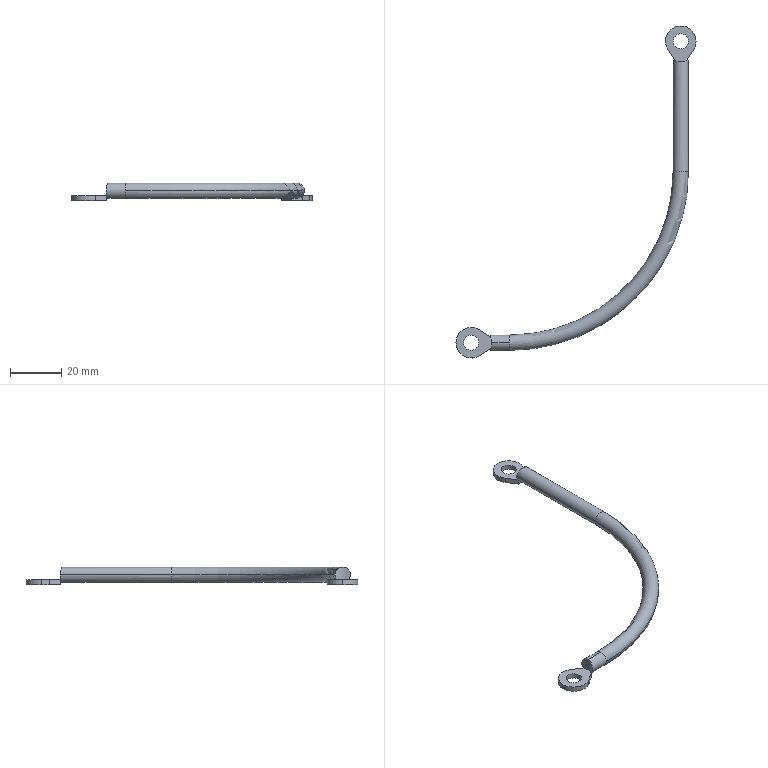Part | SolidWorks | features BaseBody 1 | 1 solid | 27 faces | box 94 x 130 x 7 mm | volume 4790 mm3 | cylinder 15 | plane 10 | torus 2 | commonest cylinder face diameters 6 x8 12 x5 16 x2
STEP:
#1=CARTESIAN_POINT('',(7.681,2.236,-4.));
#2=VERTEX_POINT('',#1);
#3=CARTESIAN_POINT('',(7.681,2.236,-2.));
#4=VERTEX_POINT('',#3);
#5=CARTESIAN_POINT('',(7.681,2.236,-15.078));
#6=DIRECTION('',(0.,0.,1.));
#7=VECTOR('',#6,1000.);
#8=LINE('',#5,#7);
#9=EDGE_CURVE('',#2,#4,#8,.T.);
#10=ORIENTED_EDGE('',*,*,#9,.F.);
#11=CARTESIAN_POINT('',(3.211,5.068,-4.));
#12=VERTEX_POINT('',#11);
#13=CARTESIAN_POINT('',(3.211,5.068,-4.));
#14=DIRECTION('',(-0.8447,0.5352,0.));
#15=VECTOR('',#14,1000.);
#16=LINE('',#13,#15);
#17=EDGE_CURVE('',#2,#12,#16,.T.);
#18=ORIENTED_EDGE('',*,*,#17,.T.);
#19=CARTESIAN_POINT('',(3.211,5.068,-2.));
#20=VERTEX_POINT('',#19);
#21=CARTESIAN_POINT('',(3.211,5.068,-15.078));
#22=DIRECTION('',(0.,0.,1.));
#23=VECTOR('',#22,1000.);
#24=LINE('',#21,#23);
#25=EDGE_CURVE('',#12,#20,#24,.T.);
#26=ORIENTED_EDGE('',*,*,#25,.T.);
#27=CARTESIAN_POINT('',(3.211,5.068,-2.));
#28=DIRECTION('',(0.8447,-0.5352,0.));
#29=VECTOR('',#28,1000.);
#30=LINE('',#27,#29);
#31=EDGE_CURVE('',#20,#4,#30,.T.);
#32=ORIENTED_EDGE('',*,*,#31,.T.);
#33=EDGE_LOOP('',(#10,#18,#26,#32));
#34=FACE_OUTER_BOUND('',#33,.T.);
#35=CARTESIAN_POINT('',(3.211,5.068,-15.078));
#36=DIRECTION('',(-0.5352,-0.8447,0.));
#37=DIRECTION('',(-0.8447,0.5352,0.));
#38=AXIS2_PLACEMENT_3D('',#35,#36,#37);
#39=PLANE('',#38);
#40=ADVANCED_FACE('',(#34),#39,.F.);
#41=CARTESIAN_POINT('',(7.681,-2.236,-2.));
#42=VERTEX_POINT('',#41);
#43=CARTESIAN_POINT('',(7.681,0.,-3.));
#44=VERTEX_POINT('',#43);
#45=CARTESIAN_POINT('',(7.681,0.,0.));
#46=DIRECTION('',(1.,0.,0.));
#47=DIRECTION('',(0.,0.,1.));
#48=AXIS2_PLACEMENT_3D('',#45,#46,#47);
#49=CIRCLE('',#48,3.);
#50=EDGE_CURVE('',#42,#44,#49,.T.);
#51=ORIENTED_EDGE('',*,*,#50,.F.);
#52=CARTESIAN_POINT('',(7.681,-2.236,-4.));
#53=VERTEX_POINT('',#52);
#54=CARTESIAN_POINT('',(7.681,-2.236,-15.078));
#55=DIRECTION('',(0.,0.,1.));
#56=VECTOR('',#55,1000.);
#57=LINE('',#54,#56);
#58=EDGE_CURVE('',#53,#42,#57,.T.);
#59=ORIENTED_EDGE('',*,*,#58,.F.);
#60=CARTESIAN_POINT('',(7.681,2.236,-4.));
#61=DIRECTION('',(0.,1.,0.));
#62=VECTOR('',#61,1000.);
#63=LINE('',#60,#62);
#64=EDGE_CURVE('',#53,#2,#63,.T.);
#65=ORIENTED_EDGE('',*,*,#64,.T.);
#66=ORIENTED_EDGE('',*,*,#9,.T.);
#67=CARTESIAN_POINT('',(7.681,0.,0.));
#68=DIRECTION('',(1.,0.,0.));
#69=DIRECTION('',(0.,0.,1.));
#70=AXIS2_PLACEMENT_3D('',#67,#68,#69);
#71=CIRCLE('',#70,3.);
#72=EDGE_CURVE('',#44,#4,#71,.T.);
#73=ORIENTED_EDGE('',*,*,#72,.F.);
#74=EDGE_LOOP('',(#51,#59,#65,#66,#73));
#75=FACE_OUTER_BOUND('',#74,.T.);
#76=CARTESIAN_POINT('',(7.681,2.236,-15.078));
#77=DIRECTION('',(-1.,0.,0.));
#78=DIRECTION('',(0.,0.,1.));
#79=AXIS2_PLACEMENT_3D('',#76,#77,#78);
#80=PLANE('',#79);
#81=ADVANCED_FACE('',(#75),#80,.F.);
#82=CARTESIAN_POINT('',(3.211,-5.068,-4.));
#83=VERTEX_POINT('',#82);
#84=CARTESIAN_POINT('',(3.211,-5.068,-2.));
#85=VERTEX_POINT('',#84);
#86=CARTESIAN_POINT('',(3.211,-5.068,-15.078));
#87=DIRECTION('',(0.,0.,1.));
#88=VECTOR('',#87,1000.);
#89=LINE('',#86,#88);
#90=EDGE_CURVE('',#83,#85,#89,.T.);
#91=ORIENTED_EDGE('',*,*,#90,.F.);
#92=CARTESIAN_POINT('',(7.681,-2.236,-4.));
#93=DIRECTION('',(0.8447,0.5352,0.));
#94=VECTOR('',#93,1000.);
#95=LINE('',#92,#94);
#96=EDGE_CURVE('',#83,#53,#95,.T.);
#97=ORIENTED_EDGE('',*,*,#96,.T.);
#98=ORIENTED_EDGE('',*,*,#58,.T.);
#99=CARTESIAN_POINT('',(7.681,-2.236,-2.));
#100=DIRECTION('',(-0.8447,-0.5352,0.));
#101=VECTOR('',#100,1000.);
#102=LINE('',#99,#101);
#103=EDGE_CURVE('',#42,#85,#102,.T.);
#104=ORIENTED_EDGE('',*,*,#103,.T.);
#105=EDGE_LOOP('',(#91,#97,#98,#104));
#106=FACE_OUTER_BOUND('',#105,.T.);
#107=CARTESIAN_POINT('',(7.681,-2.236,-15.078));
#108=DIRECTION('',(-0.5352,0.8447,0.));
#109=DIRECTION('',(0.,0.,1.));
#110=AXIS2_PLACEMENT_3D('',#107,#108,#109);
#111=PLANE('',#110);
#112=ADVANCED_FACE('',(#106),#111,.F.);
#113=CARTESIAN_POINT('',(84.236,110.319,-4.));
#114=VERTEX_POINT('',#113);
#115=CARTESIAN_POINT('',(84.236,110.319,-2.));
#116=VERTEX_POINT('',#115);
#117=CARTESIAN_POINT('',(84.236,110.319,-15.078));
#118=DIRECTION('',(0.,0.,1.));
#119=VECTOR('',#118,1000.);
#120=LINE('',#117,#119);
#121=EDGE_CURVE('',#114,#116,#120,.T.);
#122=ORIENTED_EDGE('',*,*,#121,.F.);
#123=CARTESIAN_POINT('',(87.068,114.789,-4.));
#124=VERTEX_POINT('',#123);
#125=CARTESIAN_POINT('',(87.068,114.789,-4.));
#126=DIRECTION('',(0.5352,0.8447,0.));
#127=VECTOR('',#126,1000.);
#128=LINE('',#125,#127);
#129=EDGE_CURVE('',#114,#124,#128,.T.);
#130=ORIENTED_EDGE('',*,*,#129,.T.);
#131=CARTESIAN_POINT('',(87.068,114.789,-2.));
#132=VERTEX_POINT('',#131);
#133=CARTESIAN_POINT('',(87.068,114.789,-15.078));
#134=DIRECTION('',(0.,0.,1.));
#135=VECTOR('',#134,1000.);
#136=LINE('',#133,#135);
#137=EDGE_CURVE('',#124,#132,#136,.T.);
#138=ORIENTED_EDGE('',*,*,#137,.T.);
#139=CARTESIAN_POINT('',(87.068,114.789,-2.));
#140=DIRECTION('',(-0.5352,-0.8447,0.));
#141=VECTOR('',#140,1000.);
#142=LINE('',#139,#141);
#143=EDGE_CURVE('',#132,#116,#142,.T.);
#144=ORIENTED_EDGE('',*,*,#143,.T.);
#145=EDGE_LOOP('',(#122,#130,#138,#144));
#146=FACE_OUTER_BOUND('',#145,.T.);
#147=CARTESIAN_POINT('',(87.068,114.789,-15.078));
#148=DIRECTION('',(-0.8447,0.5352,0.));
#149=DIRECTION('',(0.,0.,1.));
#150=AXIS2_PLACEMENT_3D('',#147,#148,#149);
#151=PLANE('',#150);
#152=ADVANCED_FACE('',(#146),#151,.F.);
#153=CARTESIAN_POINT('',(79.764,110.319,-2.));
#154=VERTEX_POINT('',#153);
#155=CARTESIAN_POINT('',(82.,110.319,0.));
#156=DIRECTION('',(0.,-1.,0.));
#157=DIRECTION('',(0.,0.,1.));
#158=AXIS2_PLACEMENT_3D('',#155,#156,#157);
#159=CIRCLE('',#158,3.);
#160=EDGE_CURVE('',#154,#116,#159,.T.);
#161=ORIENTED_EDGE('',*,*,#160,.F.);
#162=CARTESIAN_POINT('',(79.764,110.319,-4.));
#163=VERTEX_POINT('',#162);
#164=CARTESIAN_POINT('',(79.764,110.319,-15.078));
#165=DIRECTION('',(0.,0.,1.));
#166=VECTOR('',#165,1000.);
#167=LINE('',#164,#166);
#168=EDGE_CURVE('',#163,#154,#167,.T.);
#169=ORIENTED_EDGE('',*,*,#168,.F.);
#170=CARTESIAN_POINT('',(84.236,110.319,-4.));
#171=DIRECTION('',(1.,0.,0.));
#172=VECTOR('',#171,1000.);
#173=LINE('',#170,#172);
#174=EDGE_CURVE('',#163,#114,#173,.T.);
#175=ORIENTED_EDGE('',*,*,#174,.T.);
#176=ORIENTED_EDGE('',*,*,#121,.T.);
#177=EDGE_LOOP('',(#161,#169,#175,#176));
#178=FACE_OUTER_BOUND('',#177,.T.);
#179=CARTESIAN_POINT('',(84.236,110.319,-15.078));
#180=DIRECTION('',(0.,1.,0.));
#181=DIRECTION('',(1.,0.,0.));
#182=AXIS2_PLACEMENT_3D('',#179,#180,#181);
#183=PLANE('',#182);
#184=ADVANCED_FACE('',(#178),#183,.F.);
#185=CARTESIAN_POINT('',(76.932,114.789,-4.));
#186=VERTEX_POINT('',#185);
#187=CARTESIAN_POINT('',(76.932,114.789,-2.));
#188=VERTEX_POINT('',#187);
#189=CARTESIAN_POINT('',(76.932,114.789,-15.078));
#190=DIRECTION('',(0.,0.,1.));
#191=VECTOR('',#190,1000.);
#192=LINE('',#189,#191);
#193=EDGE_CURVE('',#186,#188,#192,.T.);
#194=ORIENTED_EDGE('',*,*,#193,.F.);
#195=CARTESIAN_POINT('',(79.764,110.319,-4.));
#196=DIRECTION('',(0.5352,-0.8447,0.));
#197=VECTOR('',#196,1000.);
#198=LINE('',#195,#197);
#199=EDGE_CURVE('',#186,#163,#198,.T.);
#200=ORIENTED_EDGE('',*,*,#199,.T.);
#201=ORIENTED_EDGE('',*,*,#168,.T.);
#202=CARTESIAN_POINT('',(79.764,110.319,-2.));
#203=DIRECTION('',(-0.5352,0.8447,0.));
#204=VECTOR('',#203,1000.);
#205=LINE('',#202,#204);
#206=EDGE_CURVE('',#154,#188,#205,.T.);
#207=ORIENTED_EDGE('',*,*,#206,.T.);
#208=EDGE_LOOP('',(#194,#200,#201,#207));
#209=FACE_OUTER_BOUND('',#208,.T.);
#210=CARTESIAN_POINT('',(79.764,110.319,-15.078));
#211=DIRECTION('',(0.8447,0.5352,0.));
#212=DIRECTION('',(0.,0.,-1.));
#213=AXIS2_PLACEMENT_3D('',#210,#211,#212);
#214=PLANE('',#213);
#215=ADVANCED_FACE('',(#209),#214,.F.);
#216=CARTESIAN_POINT('',(0.,0.,-2.));
#217=DIRECTION('',(0.,0.,1.));
#218=DIRECTION('',(1.,0.,0.));
#219=AXIS2_PLACEMENT_3D('',#216,#217,#218);
#220=CIRCLE('',#219,8.);
#221=EDGE_CURVE('',#42,#4,#220,.T.);
#222=ORIENTED_EDGE('',*,*,#221,.F.);
#223=CARTESIAN_POINT('',(8.,0.,3.));
#224=VERTEX_POINT('',#223);
#225=CARTESIAN_POINT('',(8.,0.,3.));
#226=CARTESIAN_POINT('',(8.,-0.1411,3.));
#227=CARTESIAN_POINT('',(7.996,-0.284,2.99));
#228=CARTESIAN_POINT('',(7.985,-0.499,2.959));
#229=CARTESIAN_POINT('',(7.98,-0.5708,2.946));
#230=CARTESIAN_POINT('',(7.971,-0.6783,2.923));
#231=CARTESIAN_POINT('',(7.967,-0.732,2.91));
#232=CARTESIAN_POINT('',(7.96,-0.7945,2.893));
#233=CARTESIAN_POINT('',(7.958,-0.8212,2.885));
#234=CARTESIAN_POINT('',(7.956,-0.839,2.88));
#235=CARTESIAN_POINT('',(7.955,-0.8491,2.877));
#236=CARTESIAN_POINT('',(7.941,-0.9804,2.838));
#237=CARTESIAN_POINT('',(7.924,-1.109,2.791));
#238=CARTESIAN_POINT('',(7.893,-1.305,2.702));
#239=CARTESIAN_POINT('',(7.882,-1.371,2.669));
#240=CARTESIAN_POINT('',(7.864,-1.47,2.615));
#241=CARTESIAN_POINT('',(7.854,-1.52,2.587));
#242=CARTESIAN_POINT('',(7.843,-1.578,2.551));
#243=CARTESIAN_POINT('',(7.837,-1.607,2.533));
#244=CARTESIAN_POINT('',(7.834,-1.62,2.525));
#245=CARTESIAN_POINT('',(7.833,-1.628,2.52));
#246=CARTESIAN_POINT('',(7.832,-1.633,2.516));
#247=CARTESIAN_POINT('',(7.82,-1.687,2.481));
#248=CARTESIAN_POINT('',(7.808,-1.741,2.444));
#249=CARTESIAN_POINT('',(7.789,-1.827,2.38));
#250=CARTESIAN_POINT('',(7.782,-1.856,2.357));
#251=CARTESIAN_POINT('',(7.771,-1.901,2.321));
#252=CARTESIAN_POINT('',(7.765,-1.924,2.302));
#253=CARTESIAN_POINT('',(7.76,-1.947,2.283));
#254=CARTESIAN_POINT('',(7.756,-1.962,2.27));
#255=CARTESIAN_POINT('',(7.753,-1.971,2.262));
#256=CARTESIAN_POINT('',(7.738,-2.031,2.209));
#257=CARTESIAN_POINT('',(7.717,-2.109,2.136));
#258=CARTESIAN_POINT('',(7.693,-2.195,2.046));
#259=CARTESIAN_POINT('',(7.681,-2.237,1.999));
#260=CARTESIAN_POINT('',(7.676,-2.254,1.979));
#261=CARTESIAN_POINT('',(7.672,-2.266,1.966));
#262=CARTESIAN_POINT('',(7.671,-2.271,1.96));
#263=CARTESIAN_POINT('',(7.636,-2.386,1.826));
#264=CARTESIAN_POINT('',(7.608,-2.476,1.7));
#265=CARTESIAN_POINT('',(7.57,-2.589,1.518));
#266=CARTESIAN_POINT('',(7.558,-2.622,1.459));
#267=CARTESIAN_POINT('',(7.542,-2.668,1.371));
#268=CARTESIAN_POINT('',(7.534,-2.69,1.329));
#269=CARTESIAN_POINT('',(7.526,-2.713,1.28));
#270=CARTESIAN_POINT('',(7.522,-2.723,1.259));
#271=CARTESIAN_POINT('',(7.52,-2.729,1.245));
#272=CARTESIAN_POINT('',(7.519,-2.732,1.24));
#273=CARTESIAN_POINT('',(7.495,-2.799,1.091));
#274=CARTESIAN_POINT('',(7.476,-2.849,0.9501));
#275=CARTESIAN_POINT('',(7.453,-2.908,0.7416));
#276=CARTESIAN_POINT('',(7.446,-2.924,0.6726));
#277=CARTESIAN_POINT('',(7.438,-2.946,0.5701));
#278=CARTESIAN_POINT('',(7.434,-2.955,0.5191));
#279=CARTESIAN_POINT('',(7.431,-2.963,0.4685));
#280=CARTESIAN_POINT('',(7.429,-2.968,0.435));
#281=CARTESIAN_POINT('',(7.428,-2.971,0.4194));
#282=CARTESIAN_POINT('',(7.419,-2.992,0.2582));
#283=CARTESIAN_POINT('',(7.416,-3.001,0.1133));
#284=CARTESIAN_POINT('',(7.417,-2.999,-0.1042));
#285=CARTESIAN_POINT('',(7.418,-2.996,-0.1767));
#286=CARTESIAN_POINT('',(7.422,-2.987,-0.2852));
#287=CARTESIAN_POINT('',(7.424,-2.981,-0.3393));
#288=CARTESIAN_POINT('',(7.427,-2.974,-0.3934));
#289=CARTESIAN_POINT('',(7.429,-2.969,-0.4293));
#290=CARTESIAN_POINT('',(7.43,-2.966,-0.4488));
#291=CARTESIAN_POINT('',(7.439,-2.943,-0.5972));
#292=CARTESIAN_POINT('',(7.451,-2.913,-0.733));
#293=CARTESIAN_POINT('',(7.475,-2.85,-0.94));
#294=CARTESIAN_POINT('',(7.484,-2.826,-1.009));
#295=CARTESIAN_POINT('',(7.499,-2.786,-1.114));
#296=CARTESIAN_POINT('',(7.507,-2.764,-1.166));
#297=CARTESIAN_POINT('',(7.517,-2.737,-1.228));
#298=CARTESIAN_POINT('',(7.522,-2.723,-1.258));
#299=CARTESIAN_POINT('',(7.524,-2.717,-1.271));
#300=CARTESIAN_POINT('',(7.526,-2.713,-1.28));
#301=CARTESIAN_POINT('',(7.527,-2.71,-1.286));
#302=CARTESIAN_POINT('',(7.56,-2.618,-1.48));
#303=CARTESIAN_POINT('',(7.611,-2.476,-1.732));
#304=CARTESIAN_POINT('',(7.681,-2.236,-2.));
#305=B_SPLINE_CURVE_WITH_KNOTS('',3,(#225,#226,#227,#228,#229,#230,#231,#232,#233,#234,#235,#236,#237,#238,#239,#240,#241,#242,#243,#244,#245,#246,#247,#248,#249,#250,#251,#252,#253,#254,#255,#256,#257,#258,#259,#260,#261,#262,#263,#264,#265,#266,#267,#268,#269,#270,#271,#272,#273,#274,#275,#276,#277,#278,#279,#280,#281,#282,#283,#284,#285,#286,#287,#288,#289,#290,#291,#292,#293,#294,#295,#296,#297,#298,#299,#300,#301,#302,#303,#304),.UNSPECIFIED.,.F.,.F.,(4,2,2,1,1,2,2,2,2,1,1,1,2,2,2,2,1,2,2,1,1,1,2,2,2,2,1,1,2,2,2,2,1,2,2,2,2,1,2,2,2,2,1,1,1,2,2,4),(0.,0.0625,0.09375,0.1094,0.1172,0.1211,0.125,0.1875,0.2187,0.2344,0.2422,0.2461,0.248,0.25,0.2812,0.2969,0.3047,0.3086,0.3125,0.3437,0.3594,0.3672,0.3711,0.375,0.4375,0.4687,0.4844,0.4922,0.4961,0.5,0.5625,0.5937,0.6094,0.6172,0.625,0.6875,0.7187,0.7344,0.7422,0.75,0.8125,0.8437,0.8594,0.8672,0.8711,0.873,0.875,1.),.UNSPECIFIED.);
#306=EDGE_CURVE('',#224,#42,#305,.T.);
#307=ORIENTED_EDGE('',*,*,#306,.F.);
#308=CARTESIAN_POINT('',(7.681,2.236,-2.));
#309=CARTESIAN_POINT('',(7.646,2.356,-1.866));
#310=CARTESIAN_POINT('',(7.616,2.452,-1.735));
#311=CARTESIAN_POINT('',(7.577,2.567,-1.554));
#312=CARTESIAN_POINT('',(7.566,2.601,-1.497));
#313=CARTESIAN_POINT('',(7.55,2.646,-1.415));
#314=CARTESIAN_POINT('',(7.543,2.667,-1.375));
#315=CARTESIAN_POINT('',(7.535,2.689,-1.331));
#316=CARTESIAN_POINT('',(7.531,2.699,-1.309));
#317=CARTESIAN_POINT('',(7.529,2.704,-1.3));
#318=CARTESIAN_POINT('',(7.528,2.706,-1.294));
#319=CARTESIAN_POINT('',(7.528,2.707,-1.293));
#320=CARTESIAN_POINT('',(7.503,2.776,-1.149));
#321=CARTESIAN_POINT('',(7.483,2.829,-1.009));
#322=CARTESIAN_POINT('',(7.459,2.892,-0.8019));
#323=CARTESIAN_POINT('',(7.452,2.91,-0.7335));
#324=CARTESIAN_POINT('',(7.443,2.933,-0.632));
#325=CARTESIAN_POINT('',(7.439,2.943,-0.5815));
#326=CARTESIAN_POINT('',(7.435,2.953,-0.5315));
#327=CARTESIAN_POINT('',(7.433,2.958,-0.4983));
#328=CARTESIAN_POINT('',(7.432,2.961,-0.4832));
#329=CARTESIAN_POINT('',(7.422,2.986,-0.3218));
#330=CARTESIAN_POINT('',(7.417,2.998,-0.1769));
#331=CARTESIAN_POINT('',(7.416,3.001,0.04039));
#332=CARTESIAN_POINT('',(7.417,2.999,0.1128));
#333=CARTESIAN_POINT('',(7.419,2.992,0.2211));
#334=CARTESIAN_POINT('',(7.421,2.988,0.2752));
#335=CARTESIAN_POINT('',(7.423,2.982,0.3292));
#336=CARTESIAN_POINT('',(7.425,2.978,0.3651));
#337=CARTESIAN_POINT('',(7.426,2.975,0.3842));
#338=CARTESIAN_POINT('',(7.434,2.955,0.5349));
#339=CARTESIAN_POINT('',(7.445,2.927,0.6725));
#340=CARTESIAN_POINT('',(7.468,2.868,0.8818));
#341=CARTESIAN_POINT('',(7.477,2.846,0.9521));
#342=CARTESIAN_POINT('',(7.491,2.808,1.058));
#343=CARTESIAN_POINT('',(7.499,2.787,1.111));
#344=CARTESIAN_POINT('',(7.508,2.762,1.172));
#345=CARTESIAN_POINT('',(7.513,2.748,1.203));
#346=CARTESIAN_POINT('',(7.515,2.742,1.217));
#347=CARTESIAN_POINT('',(7.517,2.738,1.225));
#348=CARTESIAN_POINT('',(7.518,2.736,1.231));
#349=CARTESIAN_POINT('',(7.535,2.689,1.334));
#350=CARTESIAN_POINT('',(7.555,2.632,1.447));
#351=CARTESIAN_POINT('',(7.593,2.52,1.63));
#352=CARTESIAN_POINT('',(7.607,2.478,1.693));
#353=CARTESIAN_POINT('',(7.629,2.408,1.79));
#354=CARTESIAN_POINT('',(7.641,2.371,1.838));
#355=CARTESIAN_POINT('',(7.655,2.325,1.896));
#356=CARTESIAN_POINT('',(7.661,2.304,1.921));
#357=CARTESIAN_POINT('',(7.665,2.29,1.938));
#358=CARTESIAN_POINT('',(7.668,2.282,1.948));
#359=CARTESIAN_POINT('',(7.697,2.183,2.062));
#360=CARTESIAN_POINT('',(7.725,2.082,2.164));
#361=CARTESIAN_POINT('',(7.766,1.923,2.304));
#362=CARTESIAN_POINT('',(7.779,1.868,2.349));
#363=CARTESIAN_POINT('',(7.799,1.782,2.413));
#364=CARTESIAN_POINT('',(7.809,1.739,2.445));
#365=CARTESIAN_POINT('',(7.818,1.695,2.475));
#366=CARTESIAN_POINT('',(7.825,1.665,2.495));
#367=CARTESIAN_POINT('',(7.828,1.652,2.504));
#368=CARTESIAN_POINT('',(7.859,1.503,2.601));
#369=CARTESIAN_POINT('',(7.883,1.37,2.673));
#370=CARTESIAN_POINT('',(7.914,1.174,2.762));
#371=CARTESIAN_POINT('',(7.923,1.109,2.788));
#372=CARTESIAN_POINT('',(7.936,1.013,2.824));
#373=CARTESIAN_POINT('',(7.942,0.9659,2.841));
#374=CARTESIAN_POINT('',(7.948,0.9112,2.858));
#375=CARTESIAN_POINT('',(7.951,0.8879,2.866));
#376=CARTESIAN_POINT('',(7.952,0.8724,2.87));
#377=CARTESIAN_POINT('',(7.953,0.8659,2.872));
#378=CARTESIAN_POINT('',(7.985,0.5721,2.96));
#379=CARTESIAN_POINT('',(8.,0.2822,3.));
#380=CARTESIAN_POINT('',(8.,0.,3.));
#381=B_SPLINE_CURVE_WITH_KNOTS('',3,(#308,#309,#310,#311,#312,#313,#314,#315,#316,#317,#318,#319,#320,#321,#322,#323,#324,#325,#326,#327,#328,#329,#330,#331,#332,#333,#334,#335,#336,#337,#338,#339,#340,#341,#342,#343,#344,#345,#346,#347,#348,#349,#350,#351,#352,#353,#354,#355,#356,#357,#358,#359,#360,#361,#362,#363,#364,#365,#366,#367,#368,#369,#370,#371,#372,#373,#374,#375,#376,#377,#378,#379,#380),.UNSPECIFIED.,.F.,.F.,(4,2,2,1,1,1,2,2,2,2,1,2,2,2,2,1,2,2,2,2,1,1,1,2,2,2,2,1,1,2,2,2,2,1,2,2,2,2,1,1,2,2,4),(0.,0.0625,0.09375,0.1094,0.1172,0.1211,0.123,0.125,0.1875,0.2188,0.2344,0.2422,0.25,0.3125,0.3438,0.3594,0.3672,0.375,0.4375,0.4688,0.4844,0.4922,0.4961,0.498,0.5,0.5625,0.5938,0.6094,0.6172,0.6211,0.625,0.6875,0.7188,0.7344,0.7422,0.75,0.8125,0.8438,0.8594,0.8672,0.8711,0.875,1.),.UNSPECIFIED.);
#382=EDGE_CURVE('',#4,#224,#381,.T.);
#383=ORIENTED_EDGE('',*,*,#382,.F.);
#384=EDGE_LOOP('',(#222,#307,#383));
#385=FACE_OUTER_BOUND('',#384,.T.);
#386=CARTESIAN_POINT('',(0.,0.,13.));
#387=DIRECTION('',(0.,0.,-1.));
#388=DIRECTION('',(-1.,0.,0.));
#389=AXIS2_PLACEMENT_3D('',#386,#387,#388);
#390=CYLINDRICAL_SURFACE('',#389,8.);
#391=ADVANCED_FACE('',(#385),#390,.F.);
#392=CARTESIAN_POINT('',(82.,118.,-2.));
#393=DIRECTION('',(0.,0.,1.));
#394=DIRECTION('',(1.,0.,0.));
#395=AXIS2_PLACEMENT_3D('',#392,#393,#394);
#396=CIRCLE('',#395,8.);
#397=EDGE_CURVE('',#154,#116,#396,.T.);
#398=ORIENTED_EDGE('',*,*,#397,.F.);
#399=CARTESIAN_POINT('',(79.,110.584,0.));
#400=VERTEX_POINT('',#399);
#401=CARTESIAN_POINT('',(79.,110.584,0.));
#402=CARTESIAN_POINT('',(79.,110.584,-0.1738));
#403=CARTESIAN_POINT('',(79.015,110.577,-0.3525));
#404=CARTESIAN_POINT('',(79.064,110.558,-0.6234));
#405=CARTESIAN_POINT('',(79.085,110.55,-0.7141));
#406=CARTESIAN_POINT('',(79.123,110.535,-0.8502));
#407=CARTESIAN_POINT('',(79.143,110.527,-0.9182));
#408=CARTESIAN_POINT('',(79.17,110.517,-0.9974));
#409=CARTESIAN_POINT('',(79.183,110.512,-1.031));
#410=CARTESIAN_POINT('',(79.191,110.509,-1.054));
#411=CARTESIAN_POINT('',(79.196,110.507,-1.067));
#412=CARTESIAN_POINT('',(79.229,110.495,-1.154));
#413=CARTESIAN_POINT('',(79.264,110.482,-1.233));
#414=CARTESIAN_POINT('',(79.323,110.461,-1.356));
#415=CARTESIAN_POINT('',(79.355,110.45,-1.417));
#416=CARTESIAN_POINT('',(79.396,110.436,-1.49));
#417=CARTESIAN_POINT('',(79.418,110.428,-1.527));
#418=CARTESIAN_POINT('',(79.427,110.425,-1.543));
#419=CARTESIAN_POINT('',(79.434,110.423,-1.553));
#420=CARTESIAN_POINT('',(79.438,110.421,-1.56));
#421=CARTESIAN_POINT('',(79.512,110.396,-1.682));
#422=CARTESIAN_POINT('',(79.615,110.362,-1.833));
#423=CARTESIAN_POINT('',(79.764,110.319,-2.));
#424=B_SPLINE_CURVE_WITH_KNOTS('',3,(#401,#402,#403,#404,#405,#406,#407,#408,#409,#410,#411,#412,#413,#414,#415,#416,#417,#418,#419,#420,#421,#422,#423),.UNSPECIFIED.,.F.,.F.,(4,2,2,1,1,2,2,2,1,1,1,2,2,4),(0.,0.25,0.375,0.4375,0.4688,0.4844,0.5,0.625,0.6875,0.7188,0.7344,0.7422,0.75,1.),.UNSPECIFIED.);
#425=EDGE_CURVE('',#400,#154,#424,.T.);
#426=ORIENTED_EDGE('',*,*,#425,.F.);
#427=CARTESIAN_POINT('',(85.,110.584,0.));
#428=VERTEX_POINT('',#427);
#429=CARTESIAN_POINT('',(85.,110.584,0.));
#430=CARTESIAN_POINT('',(85.,110.584,0.1858));
#431=CARTESIAN_POINT('',(84.983,110.576,0.3779));
#432=CARTESIAN_POINT('',(84.926,110.554,0.6697));
#433=CARTESIAN_POINT('',(84.902,110.544,0.7675));
#434=CARTESIAN_POINT('',(84.858,110.528,0.9143));
#435=CARTESIAN_POINT('',(84.834,110.519,0.9876));
#436=CARTESIAN_POINT('',(84.802,110.507,1.073));
#437=CARTESIAN_POINT('',(84.785,110.5,1.116));
#438=CARTESIAN_POINT('',(84.776,110.497,1.137));
#439=CARTESIAN_POINT('',(84.773,110.496,1.146));
#440=CARTESIAN_POINT('',(84.77,110.495,1.152));
#441=CARTESIAN_POINT('',(84.768,110.494,1.156));
#442=CARTESIAN_POINT('',(84.72,110.476,1.273));
#443=CARTESIAN_POINT('',(84.651,110.45,1.417));
#444=CARTESIAN_POINT('',(84.497,110.398,1.666));
#445=CARTESIAN_POINT('',(84.437,110.379,1.754));
#446=CARTESIAN_POINT('',(84.331,110.346,1.89));
#447=CARTESIAN_POINT('',(84.293,110.335,1.936));
#448=CARTESIAN_POINT('',(84.231,110.317,2.006));
#449=CARTESIAN_POINT('',(84.21,110.311,2.029));
#450=CARTESIAN_POINT('',(84.166,110.299,2.076));
#451=CARTESIAN_POINT('',(84.142,110.292,2.101));
#452=CARTESIAN_POINT('',(83.943,110.237,2.299));
#453=CARTESIAN_POINT('',(83.764,110.196,2.434));
#454=CARTESIAN_POINT('',(83.517,110.146,2.59));
#455=CARTESIAN_POINT('',(83.438,110.131,2.634));
#456=CARTESIAN_POINT('',(83.326,110.111,2.691));
#457=CARTESIAN_POINT('',(83.29,110.105,2.709));
#458=CARTESIAN_POINT('',(83.238,110.096,2.733));
#459=CARTESIAN_POINT('',(83.212,110.092,2.744));
#460=CARTESIAN_POINT('',(83.183,110.088,2.757));
#461=CARTESIAN_POINT('',(83.171,110.086,2.762));
#462=CARTESIAN_POINT('',(83.162,110.085,2.766));
#463=CARTESIAN_POINT('',(83.16,110.085,2.767));
#464=CARTESIAN_POINT('',(82.772,110.028,2.928));
#465=CARTESIAN_POINT('',(82.377,110.,3.));
#466=CARTESIAN_POINT('',(81.815,110.,3.));
#467=CARTESIAN_POINT('',(81.622,110.007,2.983));
#468=CARTESIAN_POINT('',(81.331,110.028,2.926));
#469=CARTESIAN_POINT('',(81.234,110.036,2.902));
#470=CARTESIAN_POINT('',(81.089,110.052,2.859));
#471=CARTESIAN_POINT('',(81.016,110.061,2.835));
#472=CARTESIAN_POINT('',(80.932,110.072,2.804));
#473=CARTESIAN_POINT('',(80.89,110.077,2.787));
#474=CARTESIAN_POINT('',(80.872,110.08,2.78));
#475=CARTESIAN_POINT('',(80.86,110.082,2.775));
#476=CARTESIAN_POINT('',(80.852,110.083,2.772));
#477=CARTESIAN_POINT('',(80.719,110.102,2.716));
#478=CARTESIAN_POINT('',(80.567,110.129,2.643));
#479=CARTESIAN_POINT('',(80.319,110.179,2.487));
#480=CARTESIAN_POINT('',(80.233,110.198,2.427));
#481=CARTESIAN_POINT('',(80.101,110.229,2.323));
#482=CARTESIAN_POINT('',(80.057,110.24,2.286));
#483=CARTESIAN_POINT('',(79.99,110.257,2.228));
#484=CARTESIAN_POINT('',(79.968,110.262,2.207));
#485=CARTESIAN_POINT('',(79.924,110.274,2.166));
#486=CARTESIAN_POINT('',(79.903,110.28,2.145));
#487=CARTESIAN_POINT('',(79.691,110.338,1.934));
#488=CARTESIAN_POINT('',(79.554,110.381,1.747));
#489=CARTESIAN_POINT('',(79.399,110.433,1.498));
#490=CARTESIAN_POINT('',(79.356,110.448,1.421));
#491=CARTESIAN_POINT('',(79.303,110.468,1.313));
#492=CARTESIAN_POINT('',(79.286,110.474,1.279));
#493=CARTESIAN_POINT('',(79.264,110.482,1.231));
#494=CARTESIAN_POINT('',(79.254,110.486,1.207));
#495=CARTESIAN_POINT('',(79.242,110.49,1.181));
#496=CARTESIAN_POINT('',(79.237,110.492,1.168));
#497=CARTESIAN_POINT('',(79.234,110.493,1.163));
#498=CARTESIAN_POINT('',(79.233,110.494,1.159));
#499=CARTESIAN_POINT('',(79.233,110.494,1.158));
#500=CARTESIAN_POINT('',(79.07,110.554,0.768));
#501=CARTESIAN_POINT('',(79.,110.584,0.3709));
#502=CARTESIAN_POINT('',(79.,110.584,0.));
#503=B_SPLINE_CURVE_WITH_KNOTS('',3,(#429,#430,#431,#432,#433,#434,#435,#436,#437,#438,#439,#440,#441,#442,#443,#444,#445,#446,#447,#448,#449,#450,#451,#452,#453,#454,#455,#456,#457,#458,#459,#460,#461,#462,#463,#464,#465,#466,#467,#468,#469,#470,#471,#472,#473,#474,#475,#476,#477,#478,#479,#480,#481,#482,#483,#484,#485,#486,#487,#488,#489,#490,#491,#492,#493,#494,#495,#496,#497,#498,#499,#500,#501,#502),.UNSPECIFIED.,.F.,.F.,(4,2,2,1,1,1,1,2,2,2,2,2,2,2,2,2,2,1,1,2,2,2,2,2,1,1,1,2,2,2,2,2,2,2,2,2,2,1,1,1,2,2,4),(0.,0.0625,0.09375,0.1094,0.1172,0.1211,0.123,0.124,0.125,0.1875,0.2187,0.2344,0.2422,0.25,0.3125,0.3437,0.3594,0.3672,0.3711,0.373,0.375,0.5,0.5625,0.5937,0.6094,0.6172,0.6211,0.623,0.625,0.6875,0.7187,0.7344,0.7422,0.75,0.8125,0.8437,0.8594,0.8672,0.8711,0.873,0.874,0.875,1.),.UNSPECIFIED.);
#504=EDGE_CURVE('',#428,#400,#503,.T.);
#505=ORIENTED_EDGE('',*,*,#504,.F.);
#506=CARTESIAN_POINT('',(84.236,110.319,-2.));
#507=CARTESIAN_POINT('',(84.31,110.34,-1.918));
#508=CARTESIAN_POINT('',(84.372,110.359,-1.839));
#509=CARTESIAN_POINT('',(84.452,110.385,-1.729));
#510=CARTESIAN_POINT('',(84.476,110.393,-1.694));
#511=CARTESIAN_POINT('',(84.51,110.404,-1.644));
#512=CARTESIAN_POINT('',(84.526,110.409,-1.619));
#513=CARTESIAN_POINT('',(84.543,110.415,-1.591));
#514=CARTESIAN_POINT('',(84.55,110.417,-1.58));
#515=CARTESIAN_POINT('',(84.555,110.419,-1.572));
#516=CARTESIAN_POINT('',(84.556,110.419,-1.57));
#517=CARTESIAN_POINT('',(84.612,110.438,-1.48));
#518=CARTESIAN_POINT('',(84.657,110.454,-1.396));
#519=CARTESIAN_POINT('',(84.717,110.475,-1.273));
#520=CARTESIAN_POINT('',(84.735,110.482,-1.233));
#521=CARTESIAN_POINT('',(84.761,110.492,-1.173));
#522=CARTESIAN_POINT('',(84.774,110.496,-1.144));
#523=CARTESIAN_POINT('',(84.785,110.5,-1.115));
#524=CARTESIAN_POINT('',(84.793,110.503,-1.095));
#525=CARTESIAN_POINT('',(84.796,110.505,-1.087));
#526=CARTESIAN_POINT('',(84.939,110.558,-0.7156));
#527=CARTESIAN_POINT('',(85.,110.584,-0.3475));
#528=CARTESIAN_POINT('',(85.,110.584,0.));
#529=B_SPLINE_CURVE_WITH_KNOTS('',3,(#506,#507,#508,#509,#510,#511,#512,#513,#514,#515,#516,#517,#518,#519,#520,#521,#522,#523,#524,#525,#526,#527,#528),.UNSPECIFIED.,.F.,.F.,(4,2,2,1,1,2,2,2,2,1,2,2,4),(0.,0.125,0.1875,0.2187,0.2344,0.2422,0.25,0.375,0.4375,0.4687,0.4844,0.5,1.),.UNSPECIFIED.);
#530=EDGE_CURVE('',#116,#428,#529,.T.);
#531=ORIENTED_EDGE('',*,*,#530,.F.);
#532=EDGE_LOOP('',(#398,#426,#505,#531));
#533=FACE_OUTER_BOUND('',#532,.T.);
#534=CARTESIAN_POINT('',(82.,118.,13.));
#535=DIRECTION('',(0.,0.,-1.));
#536=DIRECTION('',(-1.,0.,0.));
#537=AXIS2_PLACEMENT_3D('',#534,#535,#536);
#538=CYLINDRICAL_SURFACE('',#537,8.);
#539=ADVANCED_FACE('',(#533),#538,.F.);
#540=CARTESIAN_POINT('',(85.,118.,-2.));
#541=VERTEX_POINT('',#540);
#542=CARTESIAN_POINT('',(85.,118.,-4.));
#543=VERTEX_POINT('',#542);
#544=CARTESIAN_POINT('',(85.,118.,1.));
#545=DIRECTION('',(0.,0.,-1.));
#546=VECTOR('',#545,1000.);
#547=LINE('',#544,#546);
#548=EDGE_CURVE('',#541,#543,#547,.T.);
#549=ORIENTED_EDGE('',*,*,#548,.F.);
#550=CARTESIAN_POINT('',(79.,118.,-2.));
#551=VERTEX_POINT('',#550);
#552=CARTESIAN_POINT('',(82.,118.,-2.));
#553=DIRECTION('',(0.,0.,1.));
#554=DIRECTION('',(1.,0.,0.));
#555=AXIS2_PLACEMENT_3D('',#552,#553,#554);
#556=CIRCLE('',#555,3.);
#557=EDGE_CURVE('',#541,#551,#556,.T.);
#558=ORIENTED_EDGE('',*,*,#557,.T.);
#559=CARTESIAN_POINT('',(79.,118.,-4.));
#560=VERTEX_POINT('',#559);
#561=CARTESIAN_POINT('',(79.,118.,1.));
#562=DIRECTION('',(0.,0.,-1.));
#563=VECTOR('',#562,1000.);
#564=LINE('',#561,#563);
#565=EDGE_CURVE('',#551,#560,#564,.T.);
#566=ORIENTED_EDGE('',*,*,#565,.T.);
#567=CARTESIAN_POINT('',(82.,118.,-4.));
#568=DIRECTION('',(0.,0.,1.));
#569=DIRECTION('',(1.,0.,0.));
#570=AXIS2_PLACEMENT_3D('',#567,#568,#569);
#571=CIRCLE('',#570,3.);
#572=EDGE_CURVE('',#543,#560,#571,.T.);
#573=ORIENTED_EDGE('',*,*,#572,.F.);
#574=EDGE_LOOP('',(#549,#558,#566,#573));
#575=FACE_OUTER_BOUND('',#574,.T.);
#576=CARTESIAN_POINT('',(82.,118.,1.));
#577=DIRECTION('',(0.,0.,-1.));
#578=DIRECTION('',(-1.,0.,0.));
#579=AXIS2_PLACEMENT_3D('',#576,#577,#578);
#580=CYLINDRICAL_SURFACE('',#579,3.);
#581=ADVANCED_FACE('',(#575),#580,.F.);
#582=CARTESIAN_POINT('',(82.,118.,-4.));
#583=DIRECTION('',(0.,0.,1.));
#584=DIRECTION('',(1.,0.,0.));
#585=AXIS2_PLACEMENT_3D('',#582,#583,#584);
#586=CIRCLE('',#585,3.);
#587=EDGE_CURVE('',#560,#543,#586,.T.);
#588=ORIENTED_EDGE('',*,*,#587,.T.);
#589=ORIENTED_EDGE('',*,*,#572,.T.);
#590=EDGE_LOOP('',(#588,#589));
#591=FACE_BOUND('',#590,.T.);
#592=ORIENTED_EDGE('',*,*,#199,.F.);
#593=CARTESIAN_POINT('',(76.,118.,-4.));
#594=VERTEX_POINT('',#593);
#595=CARTESIAN_POINT('',(82.,118.,-4.));
#596=DIRECTION('',(0.,0.,1.));
#597=DIRECTION('',(1.,0.,0.));
#598=AXIS2_PLACEMENT_3D('',#595,#596,#597);
#599=CIRCLE('',#598,6.);
#600=EDGE_CURVE('',#594,#186,#599,.T.);
#601=ORIENTED_EDGE('',*,*,#600,.F.);
#602=CARTESIAN_POINT('',(88.,118.,-4.));
#603=VERTEX_POINT('',#602);
#604=CARTESIAN_POINT('',(82.,118.,-4.));
#605=DIRECTION('',(0.,0.,1.));
#606=DIRECTION('',(1.,0.,0.));
#607=AXIS2_PLACEMENT_3D('',#604,#605,#606);
#608=CIRCLE('',#607,6.);
#609=EDGE_CURVE('',#603,#594,#608,.T.);
#610=ORIENTED_EDGE('',*,*,#609,.F.);
#611=CARTESIAN_POINT('',(82.,118.,-4.));
#612=DIRECTION('',(0.,0.,1.));
#613=DIRECTION('',(1.,0.,0.));
#614=AXIS2_PLACEMENT_3D('',#611,#612,#613);
#615=CIRCLE('',#614,6.);
#616=EDGE_CURVE('',#124,#603,#615,.T.);
#617=ORIENTED_EDGE('',*,*,#616,.F.);
#618=ORIENTED_EDGE('',*,*,#129,.F.);
#619=ORIENTED_EDGE('',*,*,#174,.F.);
#620=EDGE_LOOP('',(#592,#601,#610,#617,#618,#619));
#621=FACE_OUTER_BOUND('',#620,.T.);
#622=CARTESIAN_POINT('',(82.,118.,-4.));
#623=DIRECTION('',(0.,0.,1.));
#624=DIRECTION('',(1.,0.,0.));
#625=AXIS2_PLACEMENT_3D('',#622,#623,#624);
#626=PLANE('',#625);
#627=ADVANCED_FACE('',(#591,#621),#626,.F.);
#628=CARTESIAN_POINT('',(82.,118.,-2.));
#629=DIRECTION('',(0.,0.,1.));
#630=DIRECTION('',(1.,0.,0.));
#631=AXIS2_PLACEMENT_3D('',#628,#629,#630);
#632=CIRCLE('',#631,3.);
#633=EDGE_CURVE('',#551,#541,#632,.T.);
#634=ORIENTED_EDGE('',*,*,#633,.F.);
#635=ORIENTED_EDGE('',*,*,#557,.F.);
#636=EDGE_LOOP('',(#634,#635));
#637=FACE_BOUND('',#636,.T.);
#638=ORIENTED_EDGE('',*,*,#397,.T.);
#639=ORIENTED_EDGE('',*,*,#143,.F.);
#640=CARTESIAN_POINT('',(88.,118.,-2.));
#641=VERTEX_POINT('',#640);
#642=CARTESIAN_POINT('',(82.,118.,-2.));
#643=DIRECTION('',(0.,0.,1.));
#644=DIRECTION('',(1.,0.,0.));
#645=AXIS2_PLACEMENT_3D('',#642,#643,#644);
#646=CIRCLE('',#645,6.);
#647=EDGE_CURVE('',#132,#641,#646,.T.);
#648=ORIENTED_EDGE('',*,*,#647,.T.);
#649=CARTESIAN_POINT('',(76.,118.,-2.));
#650=VERTEX_POINT('',#649);
#651=CARTESIAN_POINT('',(82.,118.,-2.));
#652=DIRECTION('',(0.,0.,1.));
#653=DIRECTION('',(1.,0.,0.));
#654=AXIS2_PLACEMENT_3D('',#651,#652,#653);
#655=CIRCLE('',#654,6.);
#656=EDGE_CURVE('',#641,#650,#655,.T.);
#657=ORIENTED_EDGE('',*,*,#656,.T.);
#658=CARTESIAN_POINT('',(82.,118.,-2.));
#659=DIRECTION('',(0.,0.,1.));
#660=DIRECTION('',(1.,0.,0.));
#661=AXIS2_PLACEMENT_3D('',#658,#659,#660);
#662=CIRCLE('',#661,6.);
#663=EDGE_CURVE('',#650,#188,#662,.T.);
#664=ORIENTED_EDGE('',*,*,#663,.T.);
#665=ORIENTED_EDGE('',*,*,#206,.F.);
#666=EDGE_LOOP('',(#638,#639,#648,#657,#664,#665));
#667=FACE_OUTER_BOUND('',#666,.T.);
#668=CARTESIAN_POINT('',(82.,118.,-2.));
#669=DIRECTION('',(0.,0.,1.));
#670=DIRECTION('',(1.,0.,0.));
#671=AXIS2_PLACEMENT_3D('',#668,#669,#670);
#672=PLANE('',#671);
#673=ADVANCED_FACE('',(#637,#667),#672,.T.);
#674=CARTESIAN_POINT('',(3.,0.,-2.));
#675=VERTEX_POINT('',#674);
#676=CARTESIAN_POINT('',(3.,0.,-4.));
#677=VERTEX_POINT('',#676);
#678=CARTESIAN_POINT('',(3.,0.,1.));
#679=DIRECTION('',(0.,0.,-1.));
#680=VECTOR('',#679,1000.);
#681=LINE('',#678,#680);
#682=EDGE_CURVE('',#675,#677,#681,.T.);
#683=ORIENTED_EDGE('',*,*,#682,.F.);
#684=CARTESIAN_POINT('',(-3.,0.,-2.));
#685=VERTEX_POINT('',#684);
#686=CARTESIAN_POINT('',(0.,0.,-2.));
#687=DIRECTION('',(0.,0.,1.));
#688=DIRECTION('',(1.,0.,0.));
#689=AXIS2_PLACEMENT_3D('',#686,#687,#688);
#690=CIRCLE('',#689,3.);
#691=EDGE_CURVE('',#675,#685,#690,.T.);
#692=ORIENTED_EDGE('',*,*,#691,.T.);
#693=CARTESIAN_POINT('',(-3.,0.,-4.));
#694=VERTEX_POINT('',#693);
#695=CARTESIAN_POINT('',(-3.,0.,1.));
#696=DIRECTION('',(0.,0.,-1.));
#697=VECTOR('',#696,1000.);
#698=LINE('',#695,#697);
#699=EDGE_CURVE('',#685,#694,#698,.T.);
#700=ORIENTED_EDGE('',*,*,#699,.T.);
#701=CARTESIAN_POINT('',(0.,0.,-4.));
#702=DIRECTION('',(0.,0.,1.));
#703=DIRECTION('',(1.,0.,0.));
#704=AXIS2_PLACEMENT_3D('',#701,#702,#703);
#705=CIRCLE('',#704,3.);
#706=EDGE_CURVE('',#677,#694,#705,.T.);
#707=ORIENTED_EDGE('',*,*,#706,.F.);
#708=EDGE_LOOP('',(#683,#692,#700,#707));
#709=FACE_OUTER_BOUND('',#708,.T.);
#710=CARTESIAN_POINT('',(0.,0.,1.));
#711=DIRECTION('',(0.,0.,-1.));
#712=DIRECTION('',(-1.,0.,0.));
#713=AXIS2_PLACEMENT_3D('',#710,#711,#712);
#714=CYLINDRICAL_SURFACE('',#713,3.);
#715=ADVANCED_FACE('',(#709),#714,.F.);
#716=CARTESIAN_POINT('',(0.,0.,-4.));
#717=DIRECTION('',(0.,0.,1.));
#718=DIRECTION('',(1.,0.,0.));
#719=AXIS2_PLACEMENT_3D('',#716,#717,#718);
#720=CIRCLE('',#719,3.);
#721=EDGE_CURVE('',#694,#677,#720,.T.);
#722=ORIENTED_EDGE('',*,*,#721,.T.);
#723=ORIENTED_EDGE('',*,*,#706,.T.);
#724=EDGE_LOOP('',(#722,#723));
#725=FACE_BOUND('',#724,.T.);
#726=CARTESIAN_POINT('',(-6.,0.,-4.));
#727=VERTEX_POINT('',#726);
#728=CARTESIAN_POINT('',(0.,0.,-4.));
#729=DIRECTION('',(0.,0.,1.));
#730=DIRECTION('',(1.,0.,0.));
#731=AXIS2_PLACEMENT_3D('',#728,#729,#730);
#732=CIRCLE('',#731,6.);
#733=EDGE_CURVE('',#12,#727,#732,.T.);
#734=ORIENTED_EDGE('',*,*,#733,.F.);
#735=ORIENTED_EDGE('',*,*,#17,.F.);
#736=ORIENTED_EDGE('',*,*,#64,.F.);
#737=ORIENTED_EDGE('',*,*,#96,.F.);
#738=CARTESIAN_POINT('',(0.,0.,-4.));
#739=DIRECTION('',(0.,0.,1.));
#740=DIRECTION('',(1.,0.,0.));
#741=AXIS2_PLACEMENT_3D('',#738,#739,#740);
#742=CIRCLE('',#741,6.);
#743=EDGE_CURVE('',#727,#83,#742,.T.);
#744=ORIENTED_EDGE('',*,*,#743,.F.);
#745=EDGE_LOOP('',(#734,#735,#736,#737,#744));
#746=FACE_OUTER_BOUND('',#745,.T.);
#747=CARTESIAN_POINT('',(0.,0.,-4.));
#748=DIRECTION('',(0.,0.,1.));
#749=DIRECTION('',(1.,0.,0.));
#750=AXIS2_PLACEMENT_3D('',#747,#748,#749);
#751=PLANE('',#750);
#752=ADVANCED_FACE('',(#725,#746),#751,.F.);
#753=CARTESIAN_POINT('',(0.,0.,-2.));
#754=DIRECTION('',(0.,0.,1.));
#755=DIRECTION('',(1.,0.,0.));
#756=AXIS2_PLACEMENT_3D('',#753,#754,#755);
#757=CIRCLE('',#756,3.);
#758=EDGE_CURVE('',#685,#675,#757,.T.);
#759=ORIENTED_EDGE('',*,*,#758,.F.);
#760=ORIENTED_EDGE('',*,*,#691,.F.);
#761=EDGE_LOOP('',(#759,#760));
#762=FACE_BOUND('',#761,.T.);
#763=ORIENTED_EDGE('',*,*,#221,.T.);
#764=ORIENTED_EDGE('',*,*,#31,.F.);
#765=CARTESIAN_POINT('',(-6.,0.,-2.));
#766=VERTEX_POINT('',#765);
#767=CARTESIAN_POINT('',(0.,0.,-2.));
#768=DIRECTION('',(0.,0.,1.));
#769=DIRECTION('',(1.,0.,0.));
#770=AXIS2_PLACEMENT_3D('',#767,#768,#769);
#771=CIRCLE('',#770,6.);
#772=EDGE_CURVE('',#20,#766,#771,.T.);
#773=ORIENTED_EDGE('',*,*,#772,.T.);
#774=CARTESIAN_POINT('',(0.,0.,-2.));
#775=DIRECTION('',(0.,0.,1.));
#776=DIRECTION('',(1.,0.,0.));
#777=AXIS2_PLACEMENT_3D('',#774,#775,#776);
#778=CIRCLE('',#777,6.);
#779=EDGE_CURVE('',#766,#85,#778,.T.);
#780=ORIENTED_EDGE('',*,*,#779,.T.);
#781=ORIENTED_EDGE('',*,*,#103,.F.);
#782=EDGE_LOOP('',(#763,#764,#773,#780,#781));
#783=FACE_OUTER_BOUND('',#782,.T.);
#784=CARTESIAN_POINT('',(0.,0.,-2.));
#785=DIRECTION('',(0.,0.,1.));
#786=DIRECTION('',(1.,0.,0.));
#787=AXIS2_PLACEMENT_3D('',#784,#785,#786);
#788=PLANE('',#787);
#789=ADVANCED_FACE('',(#762,#783),#788,.T.);
#790=CARTESIAN_POINT('',(15.,-3.,0.));
#791=VERTEX_POINT('',#790);
#792=CARTESIAN_POINT('',(85.,67.,0.));
#793=VERTEX_POINT('',#792);
#794=CARTESIAN_POINT('',(15.,67.,0.));
#795=DIRECTION('',(0.,0.,1.));
#796=DIRECTION('',(1.,0.,0.));
#797=AXIS2_PLACEMENT_3D('',#794,#795,#796);
#798=CIRCLE('',#797,70.);
#799=EDGE_CURVE('',#791,#793,#798,.T.);
#800=ORIENTED_EDGE('',*,*,#799,.F.);
#801=CARTESIAN_POINT('',(15.,0.,-3.));
#802=VERTEX_POINT('',#801);
#803=CARTESIAN_POINT('',(15.,0.,0.));
#804=DIRECTION('',(1.,0.,0.));
#805=DIRECTION('',(0.,0.,-1.));
#806=AXIS2_PLACEMENT_3D('',#803,#804,#805);
#807=CIRCLE('',#806,3.);
#808=EDGE_CURVE('',#791,#802,#807,.T.);
#809=ORIENTED_EDGE('',*,*,#808,.T.);
#810=CARTESIAN_POINT('',(15.,3.,0.));
#811=VERTEX_POINT('',#810);
#812=CARTESIAN_POINT('',(15.,0.,0.));
#813=DIRECTION('',(1.,0.,0.));
#814=DIRECTION('',(0.,0.,-1.));
#815=AXIS2_PLACEMENT_3D('',#812,#813,#814);
#816=CIRCLE('',#815,3.);
#817=EDGE_CURVE('',#802,#811,#816,.T.);
#818=ORIENTED_EDGE('',*,*,#817,.T.);
#819=CARTESIAN_POINT('',(79.,67.,0.));
#820=VERTEX_POINT('',#819);
#821=CARTESIAN_POINT('',(15.,67.,0.));
#822=DIRECTION('',(0.,0.,1.));
#823=DIRECTION('',(1.,0.,0.));
#824=AXIS2_PLACEMENT_3D('',#821,#822,#823);
#825=CIRCLE('',#824,64.);
#826=EDGE_CURVE('',#811,#820,#825,.T.);
#827=ORIENTED_EDGE('',*,*,#826,.T.);
#828=CARTESIAN_POINT('',(82.,67.,0.));
#829=DIRECTION('',(0.,1.,0.));
#830=DIRECTION('',(0.,0.,-1.));
#831=AXIS2_PLACEMENT_3D('',#828,#829,#830);
#832=CIRCLE('',#831,3.);
#833=EDGE_CURVE('',#793,#820,#832,.T.);
#834=ORIENTED_EDGE('',*,*,#833,.F.);
#835=EDGE_LOOP('',(#800,#809,#818,#827,#834));
#836=FACE_OUTER_BOUND('',#835,.T.);
#837=CARTESIAN_POINT('',(15.,67.,0.));
#838=DIRECTION('',(0.,0.,1.));
#839=DIRECTION('',(1.,0.,0.));
#840=AXIS2_PLACEMENT_3D('',#837,#838,#839);
#841=TOROIDAL_SURFACE('',#840,67.,3.);
#842=ADVANCED_FACE('',(#836),#841,.T.);
#843=CARTESIAN_POINT('',(88.,118.,1.));
#844=DIRECTION('',(0.,0.,-1.));
#845=VECTOR('',#844,1000.);
#846=LINE('',#843,#845);
#847=EDGE_CURVE('',#641,#603,#846,.T.);
#848=ORIENTED_EDGE('',*,*,#847,.F.);
#849=ORIENTED_EDGE('',*,*,#647,.F.);
#850=ORIENTED_EDGE('',*,*,#137,.F.);
#851=ORIENTED_EDGE('',*,*,#616,.T.);
#852=EDGE_LOOP('',(#848,#849,#850,#851));
#853=FACE_OUTER_BOUND('',#852,.T.);
#854=CARTESIAN_POINT('',(82.,118.,1.));
#855=DIRECTION('',(0.,0.,-1.));
#856=DIRECTION('',(-1.,0.,0.));
#857=AXIS2_PLACEMENT_3D('',#854,#855,#856);
#858=CYLINDRICAL_SURFACE('',#857,6.);
#859=ADVANCED_FACE('',(#853),#858,.T.);
#860=CARTESIAN_POINT('',(85.,67.,0.));
#861=DIRECTION('',(0.,1.,0.));
#862=VECTOR('',#861,1000.);
#863=LINE('',#860,#862);
#864=EDGE_CURVE('',#793,#428,#863,.T.);
#865=ORIENTED_EDGE('',*,*,#864,.F.);
#866=ORIENTED_EDGE('',*,*,#833,.T.);
#867=CARTESIAN_POINT('',(79.,67.,0.));
#868=DIRECTION('',(0.,1.,0.));
#869=VECTOR('',#868,1000.);
#870=LINE('',#867,#869);
#871=EDGE_CURVE('',#820,#400,#870,.T.);
#872=ORIENTED_EDGE('',*,*,#871,.T.);
#873=ORIENTED_EDGE('',*,*,#425,.T.);
#874=ORIENTED_EDGE('',*,*,#160,.T.);
#875=ORIENTED_EDGE('',*,*,#530,.T.);
#876=EDGE_LOOP('',(#865,#866,#872,#873,#874,#875));
#877=FACE_OUTER_BOUND('',#876,.T.);
#878=CARTESIAN_POINT('',(82.,67.,0.));
#879=DIRECTION('',(0.,1.,0.));
#880=DIRECTION('',(-1.,0.,0.));
#881=AXIS2_PLACEMENT_3D('',#878,#879,#880);
#882=CYLINDRICAL_SURFACE('',#881,3.);
#883=ADVANCED_FACE('',(#877),#882,.T.);
#884=CARTESIAN_POINT('',(-6.,0.,1.));
#885=DIRECTION('',(0.,0.,-1.));
#886=VECTOR('',#885,1000.);
#887=LINE('',#884,#886);
#888=EDGE_CURVE('',#766,#727,#887,.T.);
#889=ORIENTED_EDGE('',*,*,#888,.F.);
#890=ORIENTED_EDGE('',*,*,#772,.F.);
#891=ORIENTED_EDGE('',*,*,#25,.F.);
#892=ORIENTED_EDGE('',*,*,#733,.T.);
#893=EDGE_LOOP('',(#889,#890,#891,#892));
#894=FACE_OUTER_BOUND('',#893,.T.);
#895=CARTESIAN_POINT('',(0.,0.,1.));
#896=DIRECTION('',(0.,0.,-1.));
#897=DIRECTION('',(-1.,0.,0.));
#898=AXIS2_PLACEMENT_3D('',#895,#896,#897);
#899=CYLINDRICAL_SURFACE('',#898,6.);
#900=ADVANCED_FACE('',(#894),#899,.T.);
#901=CARTESIAN_POINT('',(15.,0.,3.));
#902=VERTEX_POINT('',#901);
#903=CARTESIAN_POINT('',(0.,0.,3.));
#904=DIRECTION('',(1.,0.,0.));
#905=VECTOR('',#904,1000.);
#906=LINE('',#903,#905);
#907=EDGE_CURVE('',#224,#902,#906,.T.);
#908=ORIENTED_EDGE('',*,*,#907,.F.);
#909=ORIENTED_EDGE('',*,*,#306,.T.);
#910=ORIENTED_EDGE('',*,*,#50,.T.);
#911=CARTESIAN_POINT('',(0.,0.,-3.));
#912=DIRECTION('',(1.,0.,0.));
#913=VECTOR('',#912,1000.);
#914=LINE('',#911,#913);
#915=EDGE_CURVE('',#44,#802,#914,.T.);
#916=ORIENTED_EDGE('',*,*,#915,.T.);
#917=ORIENTED_EDGE('',*,*,#808,.F.);
#918=CARTESIAN_POINT('',(15.,0.,0.));
#919=DIRECTION('',(1.,0.,0.));
#920=DIRECTION('',(0.,0.,-1.));
#921=AXIS2_PLACEMENT_3D('',#918,#919,#920);
#922=CIRCLE('',#921,3.);
#923=EDGE_CURVE('',#902,#791,#922,.T.);
#924=ORIENTED_EDGE('',*,*,#923,.F.);
#925=EDGE_LOOP('',(#908,#909,#910,#916,#917,#924));
#926=FACE_OUTER_BOUND('',#925,.T.);
#927=CARTESIAN_POINT('',(0.,0.,0.));
#928=DIRECTION('',(1.,0.,0.));
#929=DIRECTION('',(0.,0.,-1.));
#930=AXIS2_PLACEMENT_3D('',#927,#928,#929);
#931=CYLINDRICAL_SURFACE('',#930,3.);
#932=ADVANCED_FACE('',(#926),#931,.T.);
#933=ORIENTED_EDGE('',*,*,#382,.T.);
#934=ORIENTED_EDGE('',*,*,#907,.T.);
#935=CARTESIAN_POINT('',(15.,0.,0.));
#936=DIRECTION('',(1.,0.,0.));
#937=DIRECTION('',(0.,0.,-1.));
#938=AXIS2_PLACEMENT_3D('',#935,#936,#937);
#939=CIRCLE('',#938,3.);
#940=EDGE_CURVE('',#811,#902,#939,.T.);
#941=ORIENTED_EDGE('',*,*,#940,.F.);
#942=ORIENTED_EDGE('',*,*,#817,.F.);
#943=ORIENTED_EDGE('',*,*,#915,.F.);
#944=ORIENTED_EDGE('',*,*,#72,.T.);
#945=EDGE_LOOP('',(#933,#934,#941,#942,#943,#944));
#946=FACE_OUTER_BOUND('',#945,.T.);
#947=CARTESIAN_POINT('',(0.,0.,0.));
#948=DIRECTION('',(1.,0.,0.));
#949=DIRECTION('',(0.,0.,-1.));
#950=AXIS2_PLACEMENT_3D('',#947,#948,#949);
#951=CYLINDRICAL_SURFACE('',#950,3.);
#952=ADVANCED_FACE('',(#946),#951,.T.);
#953=ORIENTED_EDGE('',*,*,#779,.F.);
#954=ORIENTED_EDGE('',*,*,#888,.T.);
#955=ORIENTED_EDGE('',*,*,#743,.T.);
#956=ORIENTED_EDGE('',*,*,#90,.T.);
#957=EDGE_LOOP('',(#953,#954,#955,#956));
#958=FACE_OUTER_BOUND('',#957,.T.);
#959=CARTESIAN_POINT('',(0.,0.,1.));
#960=DIRECTION('',(0.,0.,-1.));
#961=DIRECTION('',(-1.,0.,0.));
#962=AXIS2_PLACEMENT_3D('',#959,#960,#961);
#963=CYLINDRICAL_SURFACE('',#962,6.);
#964=ADVANCED_FACE('',(#958),#963,.T.);
#965=CARTESIAN_POINT('',(82.,67.,0.));
#966=DIRECTION('',(0.,1.,0.));
#967=DIRECTION('',(0.,0.,-1.));
#968=AXIS2_PLACEMENT_3D('',#965,#966,#967);
#969=CIRCLE('',#968,3.);
#970=EDGE_CURVE('',#820,#793,#969,.T.);
#971=ORIENTED_EDGE('',*,*,#970,.T.);
#972=ORIENTED_EDGE('',*,*,#864,.T.);
#973=ORIENTED_EDGE('',*,*,#504,.T.);
#974=ORIENTED_EDGE('',*,*,#871,.F.);
#975=EDGE_LOOP('',(#971,#972,#973,#974));
#976=FACE_OUTER_BOUND('',#975,.T.);
#977=CARTESIAN_POINT('',(82.,67.,0.));
#978=DIRECTION('',(0.,1.,0.));
#979=DIRECTION('',(-1.,0.,0.));
#980=AXIS2_PLACEMENT_3D('',#977,#978,#979);
#981=CYLINDRICAL_SURFACE('',#980,3.);
#982=ADVANCED_FACE('',(#976),#981,.T.);
#983=ORIENTED_EDGE('',*,*,#663,.F.);
#984=CARTESIAN_POINT('',(76.,118.,1.));
#985=DIRECTION('',(0.,0.,-1.));
#986=VECTOR('',#985,1000.);
#987=LINE('',#984,#986);
#988=EDGE_CURVE('',#650,#594,#987,.T.);
#989=ORIENTED_EDGE('',*,*,#988,.T.);
#990=ORIENTED_EDGE('',*,*,#600,.T.);
#991=ORIENTED_EDGE('',*,*,#193,.T.);
#992=EDGE_LOOP('',(#983,#989,#990,#991));
#993=FACE_OUTER_BOUND('',#992,.T.);
#994=CARTESIAN_POINT('',(82.,118.,1.));
#995=DIRECTION('',(0.,0.,-1.));
#996=DIRECTION('',(-1.,0.,0.));
#997=AXIS2_PLACEMENT_3D('',#994,#995,#996);
#998=CYLINDRICAL_SURFACE('',#997,6.);
#999=ADVANCED_FACE('',(#993),#998,.T.);
#1000=ORIENTED_EDGE('',*,*,#656,.F.);
#1001=ORIENTED_EDGE('',*,*,#847,.T.);
#1002=ORIENTED_EDGE('',*,*,#609,.T.);
#1003=ORIENTED_EDGE('',*,*,#988,.F.);
#1004=EDGE_LOOP('',(#1000,#1001,#1002,#1003));
#1005=FACE_OUTER_BOUND('',#1004,.T.);
#1006=CARTESIAN_POINT('',(82.,118.,1.));
#1007=DIRECTION('',(0.,0.,-1.));
#1008=DIRECTION('',(-1.,0.,0.));
#1009=AXIS2_PLACEMENT_3D('',#1006,#1007,#1008);
#1010=CYLINDRICAL_SURFACE('',#1009,6.);
#1011=ADVANCED_FACE('',(#1005),#1010,.T.);
#1012=ORIENTED_EDGE('',*,*,#758,.T.);
#1013=ORIENTED_EDGE('',*,*,#682,.T.);
#1014=ORIENTED_EDGE('',*,*,#721,.F.);
#1015=ORIENTED_EDGE('',*,*,#699,.F.);
#1016=EDGE_LOOP('',(#1012,#1013,#1014,#1015));
#1017=FACE_OUTER_BOUND('',#1016,.T.);
#1018=CARTESIAN_POINT('',(0.,0.,1.));
#1019=DIRECTION('',(0.,0.,-1.));
#1020=DIRECTION('',(-1.,0.,0.));
#1021=AXIS2_PLACEMENT_3D('',#1018,#1019,#1020);
#1022=CYLINDRICAL_SURFACE('',#1021,3.);
#1023=ADVANCED_FACE('',(#1017),#1022,.F.);
#1024=ORIENTED_EDGE('',*,*,#633,.T.);
#1025=ORIENTED_EDGE('',*,*,#548,.T.);
#1026=ORIENTED_EDGE('',*,*,#587,.F.);
#1027=ORIENTED_EDGE('',*,*,#565,.F.);
#1028=EDGE_LOOP('',(#1024,#1025,#1026,#1027));
#1029=FACE_OUTER_BOUND('',#1028,.T.);
#1030=CARTESIAN_POINT('',(82.,118.,1.));
#1031=DIRECTION('',(0.,0.,-1.));
#1032=DIRECTION('',(-1.,0.,0.));
#1033=AXIS2_PLACEMENT_3D('',#1030,#1031,#1032);
#1034=CYLINDRICAL_SURFACE('',#1033,3.);
#1035=ADVANCED_FACE('',(#1029),#1034,.F.);
#1036=ORIENTED_EDGE('',*,*,#923,.T.);
#1037=ORIENTED_EDGE('',*,*,#799,.T.);
#1038=ORIENTED_EDGE('',*,*,#970,.F.);
#1039=ORIENTED_EDGE('',*,*,#826,.F.);
#1040=ORIENTED_EDGE('',*,*,#940,.T.);
#1041=EDGE_LOOP('',(#1036,#1037,#1038,#1039,#1040));
#1042=FACE_OUTER_BOUND('',#1041,.T.);
#1043=CARTESIAN_POINT('',(15.,67.,0.));
#1044=DIRECTION('',(0.,0.,1.));
#1045=DIRECTION('',(1.,0.,0.));
#1046=AXIS2_PLACEMENT_3D('',#1043,#1044,#1045);
#1047=TOROIDAL_SURFACE('',#1046,67.,3.);
#1048=ADVANCED_FACE('',(#1042),#1047,.T.);
#1049=CLOSED_SHELL('',(#40,#81,#112,#152,#184,#215,#391,#539,#581,#627,#673,#715,#752,#789,#842,#859,#883,#900,#932,#952,#964,#982,#999,#1011,#1023,#1035,#1048));
#1050=MANIFOLD_SOLID_BREP('',#1049);
#1051=CARTESIAN_POINT('',(0.,0.,0.));
#1052=DIRECTION('',(0.,0.,1.));
#1053=DIRECTION('',(1.,0.,0.));
#1054=AXIS2_PLACEMENT_3D('',#1051,#1052,#1053);
#1055=(LENGTH_UNIT()NAMED_UNIT(*)SI_UNIT(.MILLI.,.METRE.));
#1056=UNCERTAINTY_MEASURE_WITH_UNIT(LENGTH_MEASURE(0.00001),#1055,'','');
#1057=(NAMED_UNIT(*)PLANE_ANGLE_UNIT()SI_UNIT($,.RADIAN.));
#1058=(NAMED_UNIT(*)SI_UNIT($,.STERADIAN.)SOLID_ANGLE_UNIT());
#1059=(GEOMETRIC_REPRESENTATION_CONTEXT(3)GLOBAL_UNCERTAINTY_ASSIGNED_CONTEXT((#1056))GLOBAL_UNIT_ASSIGNED_CONTEXT((#1055,#1057,#1058))REPRESENTATION_CONTEXT('',''));
#1060=ADVANCED_BREP_SHAPE_REPRESENTATION('',(#1050,#1054),#1059);